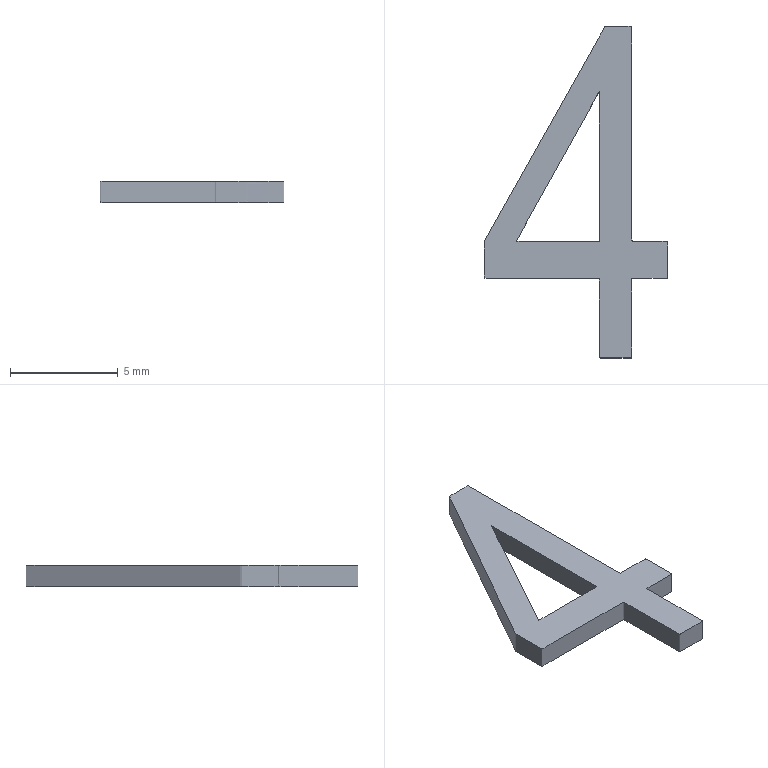Part | STEP file | lll_id1514_x_t | 1 solid | 4 faces | box 8.538 x 15.434 x 1 mm | volume 41.057 mm3 | plane 2 | other 2